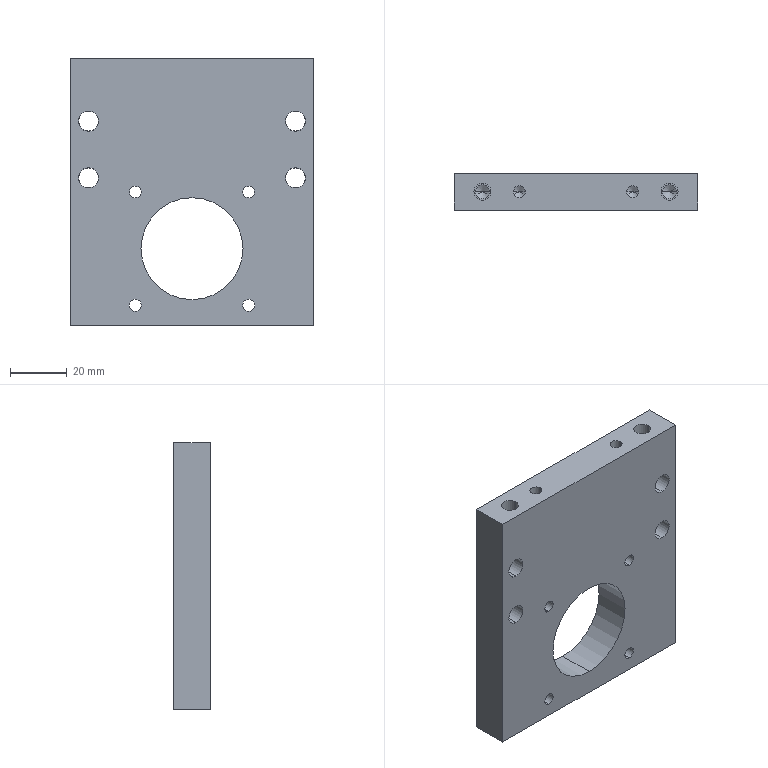Part | STEP file | OP10-120_cylinder stand (1) -L | 1 solid | 82 faces | box 86 x 13 x 94 mm | volume 86098 mm3 | cylinder 42 | cone 28 | plane 12 | commonest cylinder face diameters 4.2 x12 5 x8 7 x8 11 x8 6 x4 36 x2